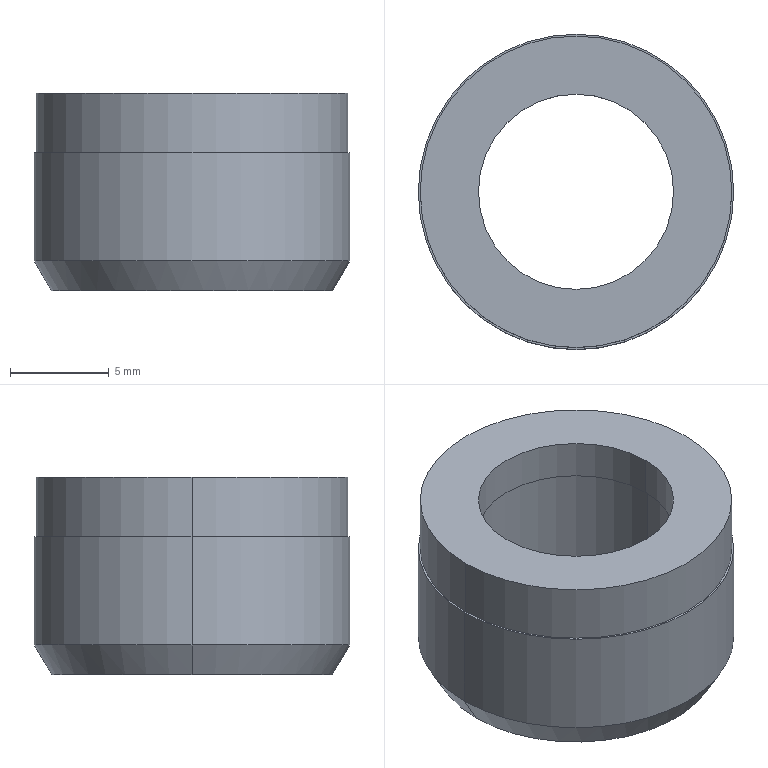Part | SolidWorks | features BaseBody 1 | 1 solid | 14 faces | box 16 x 16 x 10 mm | volume 1157 mm3 | cylinder 8 | plane 4 | cone 2 | commonest cylinder face diameters 9.9 x2 10.2 x2 15.8 x2 16 x2
STEP:
#1=CARTESIAN_POINT('',(488.537,37.715,82.366));
#2=VERTEX_POINT('',#1);
#3=CARTESIAN_POINT('',(472.537,37.715,82.366));
#4=VERTEX_POINT('',#3);
#5=CARTESIAN_POINT('',(480.537,37.715,82.366));
#6=DIRECTION('',(-0.000000013,0.,1.));
#7=DIRECTION('',(-1.,0.,-0.000000013));
#8=AXIS2_PLACEMENT_3D('',#5,#6,#7);
#9=CIRCLE('',#8,8.);
#10=EDGE_CURVE('',#2,#4,#9,.T.);
#11=ORIENTED_EDGE('',*,*,#10,.F.);
#12=CARTESIAN_POINT('',(488.537,37.715,76.866));
#13=VERTEX_POINT('',#12);
#14=CARTESIAN_POINT('',(488.537,37.715,82.366));
#15=DIRECTION('',(0.000000013,0.,-1.));
#16=VECTOR('',#15,1000.);
#17=LINE('',#14,#16);
#18=EDGE_CURVE('',#2,#13,#17,.T.);
#19=ORIENTED_EDGE('',*,*,#18,.T.);
#20=CARTESIAN_POINT('',(472.537,37.715,76.866));
#21=VERTEX_POINT('',#20);
#22=CARTESIAN_POINT('',(480.537,37.715,76.866));
#23=DIRECTION('',(0.000000013,0.,-1.));
#24=DIRECTION('',(0.,-1.,0.));
#25=AXIS2_PLACEMENT_3D('',#22,#23,#24);
#26=CIRCLE('',#25,8.);
#27=EDGE_CURVE('',#21,#13,#26,.T.);
#28=ORIENTED_EDGE('',*,*,#27,.F.);
#29=CARTESIAN_POINT('',(472.537,37.715,82.366));
#30=DIRECTION('',(0.000000013,0.,-1.));
#31=VECTOR('',#30,1000.);
#32=LINE('',#29,#31);
#33=EDGE_CURVE('',#4,#21,#32,.T.);
#34=ORIENTED_EDGE('',*,*,#33,.F.);
#35=EDGE_LOOP('',(#11,#19,#28,#34));
#36=FACE_OUTER_BOUND('',#35,.T.);
#37=CARTESIAN_POINT('',(480.537,37.715,82.366));
#38=DIRECTION('',(0.000000013,0.,-1.));
#39=DIRECTION('',(-1.,0.,-0.000000013));
#40=AXIS2_PLACEMENT_3D('',#37,#38,#39);
#41=CYLINDRICAL_SURFACE('',#40,8.);
#42=ADVANCED_FACE('',(#36),#41,.T.);
#43=CARTESIAN_POINT('',(473.403,37.715,75.366));
#44=VERTEX_POINT('',#43);
#45=CARTESIAN_POINT('',(487.671,37.715,75.366));
#46=VERTEX_POINT('',#45);
#47=CARTESIAN_POINT('',(480.537,37.715,75.366));
#48=DIRECTION('',(0.000000013,0.,-1.));
#49=DIRECTION('',(1.,0.,0.000000013));
#50=AXIS2_PLACEMENT_3D('',#47,#48,#49);
#51=CIRCLE('',#50,7.134);
#52=EDGE_CURVE('',#44,#46,#51,.T.);
#53=ORIENTED_EDGE('',*,*,#52,.F.);
#54=CARTESIAN_POINT('',(472.537,37.715,76.866));
#55=DIRECTION('',(-0.5,0.,0.866));
#56=VECTOR('',#55,1000.);
#57=LINE('',#54,#56);
#58=EDGE_CURVE('',#44,#21,#57,.T.);
#59=ORIENTED_EDGE('',*,*,#58,.T.);
#60=ORIENTED_EDGE('',*,*,#27,.T.);
#61=CARTESIAN_POINT('',(488.537,37.715,76.866));
#62=DIRECTION('',(0.5,0.,0.866));
#63=VECTOR('',#62,1000.);
#64=LINE('',#61,#63);
#65=EDGE_CURVE('',#46,#13,#64,.T.);
#66=ORIENTED_EDGE('',*,*,#65,.F.);
#67=EDGE_LOOP('',(#53,#59,#60,#66));
#68=FACE_OUTER_BOUND('',#67,.T.);
#69=CARTESIAN_POINT('',(480.537,37.715,76.866));
#70=DIRECTION('',(-0.000000013,0.,1.));
#71=DIRECTION('',(1.,0.,0.000000013));
#72=AXIS2_PLACEMENT_3D('',#69,#70,#71);
#73=CONICAL_SURFACE('',#72,8.,0.5236);
#74=ADVANCED_FACE('',(#68),#73,.T.);
#75=CARTESIAN_POINT('',(488.437,37.715,85.366));
#76=VERTEX_POINT('',#75);
#77=CARTESIAN_POINT('',(472.637,37.715,85.366));
#78=VERTEX_POINT('',#77);
#79=CARTESIAN_POINT('',(480.537,37.715,85.366));
#80=DIRECTION('',(-0.000000013,0.,1.));
#81=DIRECTION('',(-1.,0.,-0.000000013));
#82=AXIS2_PLACEMENT_3D('',#79,#80,#81);
#83=CIRCLE('',#82,7.9);
#84=EDGE_CURVE('',#76,#78,#83,.T.);
#85=ORIENTED_EDGE('',*,*,#84,.F.);
#86=CARTESIAN_POINT('',(488.437,37.715,82.366));
#87=VERTEX_POINT('',#86);
#88=CARTESIAN_POINT('',(488.437,37.715,85.366));
#89=DIRECTION('',(0.000000013,0.,-1.));
#90=VECTOR('',#89,1000.);
#91=LINE('',#88,#90);
#92=EDGE_CURVE('',#76,#87,#91,.T.);
#93=ORIENTED_EDGE('',*,*,#92,.T.);
#94=CARTESIAN_POINT('',(472.637,37.715,82.366));
#95=VERTEX_POINT('',#94);
#96=CARTESIAN_POINT('',(480.537,37.715,82.366));
#97=DIRECTION('',(-0.000000013,0.,1.));
#98=DIRECTION('',(-1.,0.,-0.000000013));
#99=AXIS2_PLACEMENT_3D('',#96,#97,#98);
#100=CIRCLE('',#99,7.9);
#101=EDGE_CURVE('',#87,#95,#100,.T.);
#102=ORIENTED_EDGE('',*,*,#101,.T.);
#103=CARTESIAN_POINT('',(472.637,37.715,85.366));
#104=DIRECTION('',(0.000000013,0.,-1.));
#105=VECTOR('',#104,1000.);
#106=LINE('',#103,#105);
#107=EDGE_CURVE('',#78,#95,#106,.T.);
#108=ORIENTED_EDGE('',*,*,#107,.F.);
#109=EDGE_LOOP('',(#85,#93,#102,#108));
#110=FACE_OUTER_BOUND('',#109,.T.);
#111=CARTESIAN_POINT('',(480.537,37.715,85.366));
#112=DIRECTION('',(0.000000013,0.,-1.));
#113=DIRECTION('',(-1.,0.,-0.000000013));
#114=AXIS2_PLACEMENT_3D('',#111,#112,#113);
#115=CYLINDRICAL_SURFACE('',#114,7.9);
#116=ADVANCED_FACE('',(#110),#115,.T.);
#117=CARTESIAN_POINT('',(475.437,37.715,83.366));
#118=VERTEX_POINT('',#117);
#119=CARTESIAN_POINT('',(485.637,37.715,83.366));
#120=VERTEX_POINT('',#119);
#121=CARTESIAN_POINT('',(480.537,37.715,83.366));
#122=DIRECTION('',(-0.000000013,0.,1.));
#123=DIRECTION('',(-1.,0.,-0.000000013));
#124=AXIS2_PLACEMENT_3D('',#121,#122,#123);
#125=CIRCLE('',#124,5.1);
#126=EDGE_CURVE('',#118,#120,#125,.T.);
#127=ORIENTED_EDGE('',*,*,#126,.T.);
#128=CARTESIAN_POINT('',(485.637,37.715,75.366));
#129=VERTEX_POINT('',#128);
#130=CARTESIAN_POINT('',(485.637,37.715,83.366));
#131=DIRECTION('',(0.000000013,0.,-1.));
#132=VECTOR('',#131,1000.);
#133=LINE('',#130,#132);
#134=EDGE_CURVE('',#120,#129,#133,.T.);
#135=ORIENTED_EDGE('',*,*,#134,.T.);
#136=CARTESIAN_POINT('',(475.437,37.715,75.366));
#137=VERTEX_POINT('',#136);
#138=CARTESIAN_POINT('',(480.537,37.715,75.366));
#139=DIRECTION('',(-0.000000013,0.,1.));
#140=DIRECTION('',(-1.,0.,-0.000000013));
#141=AXIS2_PLACEMENT_3D('',#138,#139,#140);
#142=CIRCLE('',#141,5.1);
#143=EDGE_CURVE('',#137,#129,#142,.T.);
#144=ORIENTED_EDGE('',*,*,#143,.F.);
#145=CARTESIAN_POINT('',(475.437,37.715,83.366));
#146=DIRECTION('',(0.000000013,0.,-1.));
#147=VECTOR('',#146,1000.);
#148=LINE('',#145,#147);
#149=EDGE_CURVE('',#118,#137,#148,.T.);
#150=ORIENTED_EDGE('',*,*,#149,.F.);
#151=EDGE_LOOP('',(#127,#135,#144,#150));
#152=FACE_OUTER_BOUND('',#151,.T.);
#153=CARTESIAN_POINT('',(480.537,37.715,83.366));
#154=DIRECTION('',(0.000000013,0.,-1.));
#155=DIRECTION('',(-1.,0.,-0.000000013));
#156=AXIS2_PLACEMENT_3D('',#153,#154,#155);
#157=CYLINDRICAL_SURFACE('',#156,5.1);
#158=ADVANCED_FACE('',(#152),#157,.F.);
#159=CARTESIAN_POINT('',(475.587,37.715,85.366));
#160=VERTEX_POINT('',#159);
#161=CARTESIAN_POINT('',(485.487,37.715,85.366));
#162=VERTEX_POINT('',#161);
#163=CARTESIAN_POINT('',(480.537,37.715,85.366));
#164=DIRECTION('',(-0.000000013,0.,1.));
#165=DIRECTION('',(-1.,0.,-0.000000013));
#166=AXIS2_PLACEMENT_3D('',#163,#164,#165);
#167=CIRCLE('',#166,4.95);
#168=EDGE_CURVE('',#160,#162,#167,.T.);
#169=ORIENTED_EDGE('',*,*,#168,.T.);
#170=CARTESIAN_POINT('',(485.487,37.715,83.366));
#171=VERTEX_POINT('',#170);
#172=CARTESIAN_POINT('',(485.487,37.715,85.366));
#173=DIRECTION('',(0.000000013,0.,-1.));
#174=VECTOR('',#173,1000.);
#175=LINE('',#172,#174);
#176=EDGE_CURVE('',#162,#171,#175,.T.);
#177=ORIENTED_EDGE('',*,*,#176,.T.);
#178=CARTESIAN_POINT('',(475.587,37.715,83.366));
#179=VERTEX_POINT('',#178);
#180=CARTESIAN_POINT('',(480.537,37.715,83.366));
#181=DIRECTION('',(0.000000013,0.,-1.));
#182=DIRECTION('',(-1.,0.,-0.000000013));
#183=AXIS2_PLACEMENT_3D('',#180,#181,#182);
#184=CIRCLE('',#183,4.95);
#185=EDGE_CURVE('',#171,#179,#184,.T.);
#186=ORIENTED_EDGE('',*,*,#185,.T.);
#187=CARTESIAN_POINT('',(475.587,37.715,85.366));
#188=DIRECTION('',(0.000000013,0.,-1.));
#189=VECTOR('',#188,1000.);
#190=LINE('',#187,#189);
#191=EDGE_CURVE('',#160,#179,#190,.T.);
#192=ORIENTED_EDGE('',*,*,#191,.F.);
#193=EDGE_LOOP('',(#169,#177,#186,#192));
#194=FACE_OUTER_BOUND('',#193,.T.);
#195=CARTESIAN_POINT('',(480.537,37.715,85.366));
#196=DIRECTION('',(0.000000013,0.,-1.));
#197=DIRECTION('',(-1.,0.,-0.000000013));
#198=AXIS2_PLACEMENT_3D('',#195,#196,#197);
#199=CYLINDRICAL_SURFACE('',#198,4.95);
#200=ADVANCED_FACE('',(#194),#199,.F.);
#201=ORIENTED_EDGE('',*,*,#18,.F.);
#202=CARTESIAN_POINT('',(480.537,37.715,82.366));
#203=DIRECTION('',(-0.000000013,0.,1.));
#204=DIRECTION('',(-1.,0.,-0.000000013));
#205=AXIS2_PLACEMENT_3D('',#202,#203,#204);
#206=CIRCLE('',#205,8.);
#207=EDGE_CURVE('',#4,#2,#206,.T.);
#208=ORIENTED_EDGE('',*,*,#207,.F.);
#209=ORIENTED_EDGE('',*,*,#33,.T.);
#210=CARTESIAN_POINT('',(480.537,37.715,76.866));
#211=DIRECTION('',(0.000000013,0.,-1.));
#212=DIRECTION('',(0.,-1.,0.));
#213=AXIS2_PLACEMENT_3D('',#210,#211,#212);
#214=CIRCLE('',#213,8.);
#215=EDGE_CURVE('',#13,#21,#214,.T.);
#216=ORIENTED_EDGE('',*,*,#215,.F.);
#217=EDGE_LOOP('',(#201,#208,#209,#216));
#218=FACE_OUTER_BOUND('',#217,.T.);
#219=CARTESIAN_POINT('',(480.537,37.715,82.366));
#220=DIRECTION('',(0.000000013,0.,-1.));
#221=DIRECTION('',(-1.,0.,-0.000000013));
#222=AXIS2_PLACEMENT_3D('',#219,#220,#221);
#223=CYLINDRICAL_SURFACE('',#222,8.);
#224=ADVANCED_FACE('',(#218),#223,.T.);
#225=CARTESIAN_POINT('',(480.537,37.715,82.366));
#226=DIRECTION('',(-0.000000013,0.,1.));
#227=DIRECTION('',(-1.,0.,-0.000000013));
#228=AXIS2_PLACEMENT_3D('',#225,#226,#227);
#229=CIRCLE('',#228,7.9);
#230=EDGE_CURVE('',#95,#87,#229,.T.);
#231=ORIENTED_EDGE('',*,*,#230,.F.);
#232=ORIENTED_EDGE('',*,*,#101,.F.);
#233=EDGE_LOOP('',(#231,#232));
#234=FACE_BOUND('',#233,.T.);
#235=ORIENTED_EDGE('',*,*,#207,.T.);
#236=ORIENTED_EDGE('',*,*,#10,.T.);
#237=EDGE_LOOP('',(#235,#236));
#238=FACE_OUTER_BOUND('',#237,.T.);
#239=CARTESIAN_POINT('',(488.861,46.035,82.366));
#240=DIRECTION('',(0.000000013,0.,-1.));
#241=DIRECTION('',(0.,-1.,0.));
#242=AXIS2_PLACEMENT_3D('',#239,#240,#241);
#243=PLANE('',#242);
#244=ADVANCED_FACE('',(#234,#238),#243,.F.);
#245=ORIENTED_EDGE('',*,*,#58,.F.);
#246=CARTESIAN_POINT('',(480.537,37.715,75.366));
#247=DIRECTION('',(0.000000013,0.,-1.));
#248=DIRECTION('',(1.,0.,0.000000013));
#249=AXIS2_PLACEMENT_3D('',#246,#247,#248);
#250=CIRCLE('',#249,7.134);
#251=EDGE_CURVE('',#46,#44,#250,.T.);
#252=ORIENTED_EDGE('',*,*,#251,.F.);
#253=ORIENTED_EDGE('',*,*,#65,.T.);
#254=ORIENTED_EDGE('',*,*,#215,.T.);
#255=EDGE_LOOP('',(#245,#252,#253,#254));
#256=FACE_OUTER_BOUND('',#255,.T.);
#257=CARTESIAN_POINT('',(480.537,37.715,76.866));
#258=DIRECTION('',(-0.000000013,0.,1.));
#259=DIRECTION('',(1.,0.,0.000000013));
#260=AXIS2_PLACEMENT_3D('',#257,#258,#259);
#261=CONICAL_SURFACE('',#260,8.,0.5236);
#262=ADVANCED_FACE('',(#256),#261,.T.);
#263=ORIENTED_EDGE('',*,*,#92,.F.);
#264=CARTESIAN_POINT('',(480.537,37.715,85.366));
#265=DIRECTION('',(-0.000000013,0.,1.));
#266=DIRECTION('',(-1.,0.,-0.000000013));
#267=AXIS2_PLACEMENT_3D('',#264,#265,#266);
#268=CIRCLE('',#267,7.9);
#269=EDGE_CURVE('',#78,#76,#268,.T.);
#270=ORIENTED_EDGE('',*,*,#269,.F.);
#271=ORIENTED_EDGE('',*,*,#107,.T.);
#272=ORIENTED_EDGE('',*,*,#230,.T.);
#273=EDGE_LOOP('',(#263,#270,#271,#272));
#274=FACE_OUTER_BOUND('',#273,.T.);
#275=CARTESIAN_POINT('',(480.537,37.715,85.366));
#276=DIRECTION('',(0.000000013,0.,-1.));
#277=DIRECTION('',(-1.,0.,-0.000000013));
#278=AXIS2_PLACEMENT_3D('',#275,#276,#277);
#279=CYLINDRICAL_SURFACE('',#278,7.9);
#280=ADVANCED_FACE('',(#274),#279,.T.);
#281=ORIENTED_EDGE('',*,*,#143,.T.);
#282=CARTESIAN_POINT('',(480.537,37.715,75.366));
#283=DIRECTION('',(-0.000000013,0.,1.));
#284=DIRECTION('',(-1.,0.,-0.000000013));
#285=AXIS2_PLACEMENT_3D('',#282,#283,#284);
#286=CIRCLE('',#285,5.1);
#287=EDGE_CURVE('',#129,#137,#286,.T.);
#288=ORIENTED_EDGE('',*,*,#287,.T.);
#289=EDGE_LOOP('',(#281,#288));
#290=FACE_BOUND('',#289,.T.);
#291=ORIENTED_EDGE('',*,*,#251,.T.);
#292=ORIENTED_EDGE('',*,*,#52,.T.);
#293=EDGE_LOOP('',(#291,#292));
#294=FACE_OUTER_BOUND('',#293,.T.);
#295=CARTESIAN_POINT('',(487.956,45.134,75.366));
#296=DIRECTION('',(0.000000013,0.,-1.));
#297=DIRECTION('',(0.,-1.,0.));
#298=AXIS2_PLACEMENT_3D('',#295,#296,#297);
#299=PLANE('',#298);
#300=ADVANCED_FACE('',(#290,#294),#299,.T.);
#301=ORIENTED_EDGE('',*,*,#168,.F.);
#302=CARTESIAN_POINT('',(480.537,37.715,85.366));
#303=DIRECTION('',(-0.000000013,0.,1.));
#304=DIRECTION('',(-1.,0.,-0.000000013));
#305=AXIS2_PLACEMENT_3D('',#302,#303,#304);
#306=CIRCLE('',#305,4.95);
#307=EDGE_CURVE('',#162,#160,#306,.T.);
#308=ORIENTED_EDGE('',*,*,#307,.F.);
#309=EDGE_LOOP('',(#301,#308));
#310=FACE_BOUND('',#309,.T.);
#311=ORIENTED_EDGE('',*,*,#269,.T.);
#312=ORIENTED_EDGE('',*,*,#84,.T.);
#313=EDGE_LOOP('',(#311,#312));
#314=FACE_OUTER_BOUND('',#313,.T.);
#315=CARTESIAN_POINT('',(488.757,45.931,85.366));
#316=DIRECTION('',(0.000000013,0.,-1.));
#317=DIRECTION('',(0.,-1.,0.));
#318=AXIS2_PLACEMENT_3D('',#315,#316,#317);
#319=PLANE('',#318);
#320=ADVANCED_FACE('',(#310,#314),#319,.F.);
#321=ORIENTED_EDGE('',*,*,#134,.F.);
#322=CARTESIAN_POINT('',(480.537,37.715,83.366));
#323=DIRECTION('',(-0.000000013,0.,1.));
#324=DIRECTION('',(-1.,0.,-0.000000013));
#325=AXIS2_PLACEMENT_3D('',#322,#323,#324);
#326=CIRCLE('',#325,5.1);
#327=EDGE_CURVE('',#120,#118,#326,.T.);
#328=ORIENTED_EDGE('',*,*,#327,.T.);
#329=ORIENTED_EDGE('',*,*,#149,.T.);
#330=ORIENTED_EDGE('',*,*,#287,.F.);
#331=EDGE_LOOP('',(#321,#328,#329,#330));
#332=FACE_OUTER_BOUND('',#331,.T.);
#333=CARTESIAN_POINT('',(480.537,37.715,83.366));
#334=DIRECTION('',(0.000000013,0.,-1.));
#335=DIRECTION('',(-1.,0.,-0.000000013));
#336=AXIS2_PLACEMENT_3D('',#333,#334,#335);
#337=CYLINDRICAL_SURFACE('',#336,5.1);
#338=ADVANCED_FACE('',(#332),#337,.F.);
#339=ORIENTED_EDGE('',*,*,#176,.F.);
#340=ORIENTED_EDGE('',*,*,#307,.T.);
#341=ORIENTED_EDGE('',*,*,#191,.T.);
#342=CARTESIAN_POINT('',(480.537,37.715,83.366));
#343=DIRECTION('',(0.000000013,0.,-1.));
#344=DIRECTION('',(-1.,0.,-0.000000013));
#345=AXIS2_PLACEMENT_3D('',#342,#343,#344);
#346=CIRCLE('',#345,4.95);
#347=EDGE_CURVE('',#179,#171,#346,.T.);
#348=ORIENTED_EDGE('',*,*,#347,.T.);
#349=EDGE_LOOP('',(#339,#340,#341,#348));
#350=FACE_OUTER_BOUND('',#349,.T.);
#351=CARTESIAN_POINT('',(480.537,37.715,85.366));
#352=DIRECTION('',(0.000000013,0.,-1.));
#353=DIRECTION('',(-1.,0.,-0.000000013));
#354=AXIS2_PLACEMENT_3D('',#351,#352,#353);
#355=CYLINDRICAL_SURFACE('',#354,4.95);
#356=ADVANCED_FACE('',(#350),#355,.F.);
#357=ORIENTED_EDGE('',*,*,#347,.F.);
#358=ORIENTED_EDGE('',*,*,#185,.F.);
#359=EDGE_LOOP('',(#357,#358));
#360=FACE_BOUND('',#359,.T.);
#361=ORIENTED_EDGE('',*,*,#126,.F.);
#362=ORIENTED_EDGE('',*,*,#327,.F.);
#363=EDGE_LOOP('',(#361,#362));
#364=FACE_OUTER_BOUND('',#363,.T.);
#365=CARTESIAN_POINT('',(485.845,43.019,83.366));
#366=DIRECTION('',(0.000000013,0.,-1.));
#367=DIRECTION('',(0.,-1.,0.));
#368=AXIS2_PLACEMENT_3D('',#365,#366,#367);
#369=PLANE('',#368);
#370=ADVANCED_FACE('',(#360,#364),#369,.T.);
#371=CLOSED_SHELL('',(#42,#74,#116,#158,#200,#224,#244,#262,#280,#300,#320,#338,#356,#370));
#372=MANIFOLD_SOLID_BREP('',#371);
#373=CARTESIAN_POINT('',(0.,0.,0.));
#374=DIRECTION('',(0.,0.,1.));
#375=DIRECTION('',(1.,0.,0.));
#376=AXIS2_PLACEMENT_3D('',#373,#374,#375);
#377=(LENGTH_UNIT()NAMED_UNIT(*)SI_UNIT(.MILLI.,.METRE.));
#378=UNCERTAINTY_MEASURE_WITH_UNIT(LENGTH_MEASURE(0.00001),#377,'','');
#379=(NAMED_UNIT(*)PLANE_ANGLE_UNIT()SI_UNIT($,.RADIAN.));
#380=(NAMED_UNIT(*)SI_UNIT($,.STERADIAN.)SOLID_ANGLE_UNIT());
#381=(GEOMETRIC_REPRESENTATION_CONTEXT(3)GLOBAL_UNCERTAINTY_ASSIGNED_CONTEXT((#378))GLOBAL_UNIT_ASSIGNED_CONTEXT((#377,#379,#380))REPRESENTATION_CONTEXT('',''));
#382=ADVANCED_BREP_SHAPE_REPRESENTATION('',(#372,#376),#381);